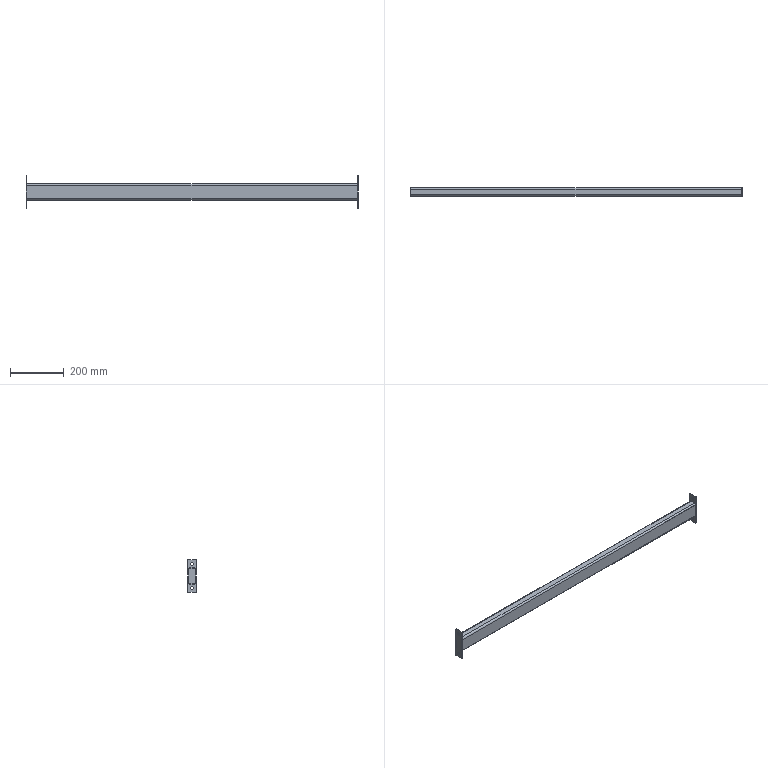Part | SolidWorks | features ICE 1, MirrorSolid 1, WeldMemberFeat 1, WeldmentFeature 1 | 3 solids | 38 faces | box 1240 x 30 x 120 mm | volume 613897 mm3 | plane 22 | cylinder 16 | commonest cylinder face diameters 10.5 x8 6 x4 12 x4
STEP:
#1=CARTESIAN_POINT('',(-617.,15.,24.));
#2=VERTEX_POINT('',#1);
#3=CARTESIAN_POINT('',(-617.,9.,30.));
#4=VERTEX_POINT('',#3);
#5=CARTESIAN_POINT('',(-617.,9.,24.));
#6=DIRECTION('',(1.,0.,0.));
#7=DIRECTION('',(0.,0.,-1.));
#8=AXIS2_PLACEMENT_3D('',#5,#6,#7);
#9=CIRCLE('',#8,6.);
#10=EDGE_CURVE('',#2,#4,#9,.T.);
#11=ORIENTED_EDGE('',*,*,#10,.T.);
#12=CARTESIAN_POINT('',(617.,9.,30.));
#13=VERTEX_POINT('',#12);
#14=CARTESIAN_POINT('',(617.,9.,30.));
#15=DIRECTION('',(-1.,0.,0.));
#16=VECTOR('',#15,1000.);
#17=LINE('',#14,#16);
#18=EDGE_CURVE('',#13,#4,#17,.T.);
#19=ORIENTED_EDGE('',*,*,#18,.F.);
#20=CARTESIAN_POINT('',(617.,15.,24.));
#21=VERTEX_POINT('',#20);
#22=CARTESIAN_POINT('',(617.,9.,24.));
#23=DIRECTION('',(1.,0.,0.));
#24=DIRECTION('',(0.,0.,-1.));
#25=AXIS2_PLACEMENT_3D('',#22,#23,#24);
#26=CIRCLE('',#25,6.);
#27=EDGE_CURVE('',#21,#13,#26,.T.);
#28=ORIENTED_EDGE('',*,*,#27,.F.);
#29=CARTESIAN_POINT('',(617.,15.,24.));
#30=DIRECTION('',(-1.,0.,0.));
#31=VECTOR('',#30,1000.);
#32=LINE('',#29,#31);
#33=EDGE_CURVE('',#21,#2,#32,.T.);
#34=ORIENTED_EDGE('',*,*,#33,.T.);
#35=EDGE_LOOP('',(#11,#19,#28,#34));
#36=FACE_OUTER_BOUND('',#35,.T.);
#37=CARTESIAN_POINT('',(617.,9.,24.));
#38=DIRECTION('',(-1.,0.,0.));
#39=DIRECTION('',(0.,0.,1.));
#40=AXIS2_PLACEMENT_3D('',#37,#38,#39);
#41=CYLINDRICAL_SURFACE('',#40,6.);
#42=ADVANCED_FACE('',(#36),#41,.T.);
#43=CARTESIAN_POINT('',(-617.,-9.,30.));
#44=VERTEX_POINT('',#43);
#45=CARTESIAN_POINT('',(-617.,9.,30.));
#46=DIRECTION('',(0.,-1.,0.));
#47=VECTOR('',#46,1000.);
#48=LINE('',#45,#47);
#49=EDGE_CURVE('',#4,#44,#48,.T.);
#50=ORIENTED_EDGE('',*,*,#49,.T.);
#51=CARTESIAN_POINT('',(617.,-9.,30.));
#52=VERTEX_POINT('',#51);
#53=CARTESIAN_POINT('',(617.,-9.,30.));
#54=DIRECTION('',(-1.,0.,0.));
#55=VECTOR('',#54,1000.);
#56=LINE('',#53,#55);
#57=EDGE_CURVE('',#52,#44,#56,.T.);
#58=ORIENTED_EDGE('',*,*,#57,.F.);
#59=CARTESIAN_POINT('',(617.,9.,30.));
#60=DIRECTION('',(0.,-1.,0.));
#61=VECTOR('',#60,1000.);
#62=LINE('',#59,#61);
#63=EDGE_CURVE('',#13,#52,#62,.T.);
#64=ORIENTED_EDGE('',*,*,#63,.F.);
#65=ORIENTED_EDGE('',*,*,#18,.T.);
#66=EDGE_LOOP('',(#50,#58,#64,#65));
#67=FACE_OUTER_BOUND('',#66,.T.);
#68=CARTESIAN_POINT('',(617.,9.,30.));
#69=DIRECTION('',(0.,0.,-1.));
#70=DIRECTION('',(-1.,0.,0.));
#71=AXIS2_PLACEMENT_3D('',#68,#69,#70);
#72=PLANE('',#71);
#73=ADVANCED_FACE('',(#67),#72,.F.);
#74=CARTESIAN_POINT('',(-617.,-15.,24.));
#75=VERTEX_POINT('',#74);
#76=CARTESIAN_POINT('',(-617.,-9.,24.));
#77=DIRECTION('',(1.,0.,0.));
#78=DIRECTION('',(0.,0.,-1.));
#79=AXIS2_PLACEMENT_3D('',#76,#77,#78);
#80=CIRCLE('',#79,6.);
#81=EDGE_CURVE('',#44,#75,#80,.T.);
#82=ORIENTED_EDGE('',*,*,#81,.T.);
#83=CARTESIAN_POINT('',(617.,-15.,24.));
#84=VERTEX_POINT('',#83);
#85=CARTESIAN_POINT('',(617.,-15.,24.));
#86=DIRECTION('',(-1.,0.,0.));
#87=VECTOR('',#86,1000.);
#88=LINE('',#85,#87);
#89=EDGE_CURVE('',#84,#75,#88,.T.);
#90=ORIENTED_EDGE('',*,*,#89,.F.);
#91=CARTESIAN_POINT('',(617.,-9.,24.));
#92=DIRECTION('',(1.,0.,0.));
#93=DIRECTION('',(0.,0.,-1.));
#94=AXIS2_PLACEMENT_3D('',#91,#92,#93);
#95=CIRCLE('',#94,6.);
#96=EDGE_CURVE('',#52,#84,#95,.T.);
#97=ORIENTED_EDGE('',*,*,#96,.F.);
#98=ORIENTED_EDGE('',*,*,#57,.T.);
#99=EDGE_LOOP('',(#82,#90,#97,#98));
#100=FACE_OUTER_BOUND('',#99,.T.);
#101=CARTESIAN_POINT('',(617.,-9.,24.));
#102=DIRECTION('',(-1.,0.,0.));
#103=DIRECTION('',(0.,0.,1.));
#104=AXIS2_PLACEMENT_3D('',#101,#102,#103);
#105=CYLINDRICAL_SURFACE('',#104,6.);
#106=ADVANCED_FACE('',(#100),#105,.T.);
#107=CARTESIAN_POINT('',(-617.,-15.,-24.));
#108=VERTEX_POINT('',#107);
#109=CARTESIAN_POINT('',(-617.,-15.,-24.));
#110=DIRECTION('',(0.,0.,-1.));
#111=VECTOR('',#110,1000.);
#112=LINE('',#109,#111);
#113=EDGE_CURVE('',#75,#108,#112,.T.);
#114=ORIENTED_EDGE('',*,*,#113,.T.);
#115=CARTESIAN_POINT('',(617.,-15.,-24.));
#116=VERTEX_POINT('',#115);
#117=CARTESIAN_POINT('',(617.,-15.,-24.));
#118=DIRECTION('',(-1.,0.,0.));
#119=VECTOR('',#118,1000.);
#120=LINE('',#117,#119);
#121=EDGE_CURVE('',#116,#108,#120,.T.);
#122=ORIENTED_EDGE('',*,*,#121,.F.);
#123=CARTESIAN_POINT('',(617.,-15.,-24.));
#124=DIRECTION('',(0.,0.,-1.));
#125=VECTOR('',#124,1000.);
#126=LINE('',#123,#125);
#127=EDGE_CURVE('',#84,#116,#126,.T.);
#128=ORIENTED_EDGE('',*,*,#127,.F.);
#129=ORIENTED_EDGE('',*,*,#89,.T.);
#130=EDGE_LOOP('',(#114,#122,#128,#129));
#131=FACE_OUTER_BOUND('',#130,.T.);
#132=CARTESIAN_POINT('',(617.,-15.,-24.));
#133=DIRECTION('',(0.,1.,0.));
#134=DIRECTION('',(0.,0.,1.));
#135=AXIS2_PLACEMENT_3D('',#132,#133,#134);
#136=PLANE('',#135);
#137=ADVANCED_FACE('',(#131),#136,.F.);
#138=CARTESIAN_POINT('',(-617.,-9.,-30.));
#139=VERTEX_POINT('',#138);
#140=CARTESIAN_POINT('',(-617.,-9.,-24.));
#141=DIRECTION('',(1.,0.,0.));
#142=DIRECTION('',(0.,0.,-1.));
#143=AXIS2_PLACEMENT_3D('',#140,#141,#142);
#144=CIRCLE('',#143,6.);
#145=EDGE_CURVE('',#108,#139,#144,.T.);
#146=ORIENTED_EDGE('',*,*,#145,.T.);
#147=CARTESIAN_POINT('',(617.,-9.,-30.));
#148=VERTEX_POINT('',#147);
#149=CARTESIAN_POINT('',(617.,-9.,-30.));
#150=DIRECTION('',(-1.,0.,0.));
#151=VECTOR('',#150,1000.);
#152=LINE('',#149,#151);
#153=EDGE_CURVE('',#148,#139,#152,.T.);
#154=ORIENTED_EDGE('',*,*,#153,.F.);
#155=CARTESIAN_POINT('',(617.,-9.,-24.));
#156=DIRECTION('',(1.,0.,0.));
#157=DIRECTION('',(0.,0.,-1.));
#158=AXIS2_PLACEMENT_3D('',#155,#156,#157);
#159=CIRCLE('',#158,6.);
#160=EDGE_CURVE('',#116,#148,#159,.T.);
#161=ORIENTED_EDGE('',*,*,#160,.F.);
#162=ORIENTED_EDGE('',*,*,#121,.T.);
#163=EDGE_LOOP('',(#146,#154,#161,#162));
#164=FACE_OUTER_BOUND('',#163,.T.);
#165=CARTESIAN_POINT('',(617.,-9.,-24.));
#166=DIRECTION('',(-1.,0.,0.));
#167=DIRECTION('',(0.,0.,1.));
#168=AXIS2_PLACEMENT_3D('',#165,#166,#167);
#169=CYLINDRICAL_SURFACE('',#168,6.);
#170=ADVANCED_FACE('',(#164),#169,.T.);
#171=CARTESIAN_POINT('',(-617.,9.,-30.));
#172=VERTEX_POINT('',#171);
#173=CARTESIAN_POINT('',(-617.,-9.,-30.));
#174=DIRECTION('',(0.,1.,0.));
#175=VECTOR('',#174,1000.);
#176=LINE('',#173,#175);
#177=EDGE_CURVE('',#139,#172,#176,.T.);
#178=ORIENTED_EDGE('',*,*,#177,.T.);
#179=CARTESIAN_POINT('',(617.,9.,-30.));
#180=VERTEX_POINT('',#179);
#181=CARTESIAN_POINT('',(617.,9.,-30.));
#182=DIRECTION('',(-1.,0.,0.));
#183=VECTOR('',#182,1000.);
#184=LINE('',#181,#183);
#185=EDGE_CURVE('',#180,#172,#184,.T.);
#186=ORIENTED_EDGE('',*,*,#185,.F.);
#187=CARTESIAN_POINT('',(617.,-9.,-30.));
#188=DIRECTION('',(0.,1.,0.));
#189=VECTOR('',#188,1000.);
#190=LINE('',#187,#189);
#191=EDGE_CURVE('',#148,#180,#190,.T.);
#192=ORIENTED_EDGE('',*,*,#191,.F.);
#193=ORIENTED_EDGE('',*,*,#153,.T.);
#194=EDGE_LOOP('',(#178,#186,#192,#193));
#195=FACE_OUTER_BOUND('',#194,.T.);
#196=CARTESIAN_POINT('',(617.,-9.,-30.));
#197=DIRECTION('',(0.,0.,1.));
#198=DIRECTION('',(1.,0.,0.));
#199=AXIS2_PLACEMENT_3D('',#196,#197,#198);
#200=PLANE('',#199);
#201=ADVANCED_FACE('',(#195),#200,.F.);
#202=CARTESIAN_POINT('',(-617.,15.,-24.));
#203=VERTEX_POINT('',#202);
#204=CARTESIAN_POINT('',(-617.,9.,-24.));
#205=DIRECTION('',(1.,0.,0.));
#206=DIRECTION('',(0.,0.,-1.));
#207=AXIS2_PLACEMENT_3D('',#204,#205,#206);
#208=CIRCLE('',#207,6.);
#209=EDGE_CURVE('',#172,#203,#208,.T.);
#210=ORIENTED_EDGE('',*,*,#209,.T.);
#211=CARTESIAN_POINT('',(617.,15.,-24.));
#212=VERTEX_POINT('',#211);
#213=CARTESIAN_POINT('',(617.,15.,-24.));
#214=DIRECTION('',(-1.,0.,0.));
#215=VECTOR('',#214,1000.);
#216=LINE('',#213,#215);
#217=EDGE_CURVE('',#212,#203,#216,.T.);
#218=ORIENTED_EDGE('',*,*,#217,.F.);
#219=CARTESIAN_POINT('',(617.,9.,-24.));
#220=DIRECTION('',(1.,0.,0.));
#221=DIRECTION('',(0.,0.,-1.));
#222=AXIS2_PLACEMENT_3D('',#219,#220,#221);
#223=CIRCLE('',#222,6.);
#224=EDGE_CURVE('',#180,#212,#223,.T.);
#225=ORIENTED_EDGE('',*,*,#224,.F.);
#226=ORIENTED_EDGE('',*,*,#185,.T.);
#227=EDGE_LOOP('',(#210,#218,#225,#226));
#228=FACE_OUTER_BOUND('',#227,.T.);
#229=CARTESIAN_POINT('',(617.,9.,-24.));
#230=DIRECTION('',(-1.,0.,0.));
#231=DIRECTION('',(0.,0.,1.));
#232=AXIS2_PLACEMENT_3D('',#229,#230,#231);
#233=CYLINDRICAL_SURFACE('',#232,6.);
#234=ADVANCED_FACE('',(#228),#233,.T.);
#235=CARTESIAN_POINT('',(-617.,-9.,27.));
#236=VERTEX_POINT('',#235);
#237=CARTESIAN_POINT('',(-617.,-12.,24.));
#238=VERTEX_POINT('',#237);
#239=CARTESIAN_POINT('',(-617.,-9.,24.));
#240=DIRECTION('',(1.,0.,0.));
#241=DIRECTION('',(0.,0.,-1.));
#242=AXIS2_PLACEMENT_3D('',#239,#240,#241);
#243=CIRCLE('',#242,3.);
#244=EDGE_CURVE('',#236,#238,#243,.T.);
#245=ORIENTED_EDGE('',*,*,#244,.F.);
#246=CARTESIAN_POINT('',(617.,-9.,27.));
#247=VERTEX_POINT('',#246);
#248=CARTESIAN_POINT('',(617.,-9.,27.));
#249=DIRECTION('',(-1.,0.,0.));
#250=VECTOR('',#249,1000.);
#251=LINE('',#248,#250);
#252=EDGE_CURVE('',#247,#236,#251,.T.);
#253=ORIENTED_EDGE('',*,*,#252,.F.);
#254=CARTESIAN_POINT('',(617.,-12.,24.));
#255=VERTEX_POINT('',#254);
#256=CARTESIAN_POINT('',(617.,-9.,24.));
#257=DIRECTION('',(1.,0.,0.));
#258=DIRECTION('',(0.,0.,-1.));
#259=AXIS2_PLACEMENT_3D('',#256,#257,#258);
#260=CIRCLE('',#259,3.);
#261=EDGE_CURVE('',#247,#255,#260,.T.);
#262=ORIENTED_EDGE('',*,*,#261,.T.);
#263=CARTESIAN_POINT('',(617.,-12.,24.));
#264=DIRECTION('',(-1.,0.,0.));
#265=VECTOR('',#264,1000.);
#266=LINE('',#263,#265);
#267=EDGE_CURVE('',#255,#238,#266,.T.);
#268=ORIENTED_EDGE('',*,*,#267,.T.);
#269=EDGE_LOOP('',(#245,#253,#262,#268));
#270=FACE_OUTER_BOUND('',#269,.T.);
#271=CARTESIAN_POINT('',(617.,-9.,24.));
#272=DIRECTION('',(-1.,0.,0.));
#273=DIRECTION('',(0.,0.,1.));
#274=AXIS2_PLACEMENT_3D('',#271,#272,#273);
#275=CYLINDRICAL_SURFACE('',#274,3.);
#276=ADVANCED_FACE('',(#270),#275,.F.);
#277=CARTESIAN_POINT('',(-617.,9.,27.));
#278=VERTEX_POINT('',#277);
#279=CARTESIAN_POINT('',(-617.,9.,27.));
#280=DIRECTION('',(0.,-1.,0.));
#281=VECTOR('',#280,1000.);
#282=LINE('',#279,#281);
#283=EDGE_CURVE('',#278,#236,#282,.T.);
#284=ORIENTED_EDGE('',*,*,#283,.F.);
#285=CARTESIAN_POINT('',(617.,9.,27.));
#286=VERTEX_POINT('',#285);
#287=CARTESIAN_POINT('',(617.,9.,27.));
#288=DIRECTION('',(-1.,0.,0.));
#289=VECTOR('',#288,1000.);
#290=LINE('',#287,#289);
#291=EDGE_CURVE('',#286,#278,#290,.T.);
#292=ORIENTED_EDGE('',*,*,#291,.F.);
#293=CARTESIAN_POINT('',(617.,9.,27.));
#294=DIRECTION('',(0.,-1.,0.));
#295=VECTOR('',#294,1000.);
#296=LINE('',#293,#295);
#297=EDGE_CURVE('',#286,#247,#296,.T.);
#298=ORIENTED_EDGE('',*,*,#297,.T.);
#299=ORIENTED_EDGE('',*,*,#252,.T.);
#300=EDGE_LOOP('',(#284,#292,#298,#299));
#301=FACE_OUTER_BOUND('',#300,.T.);
#302=CARTESIAN_POINT('',(617.,9.,27.));
#303=DIRECTION('',(0.,0.,-1.));
#304=DIRECTION('',(-1.,0.,0.));
#305=AXIS2_PLACEMENT_3D('',#302,#303,#304);
#306=PLANE('',#305);
#307=ADVANCED_FACE('',(#301),#306,.T.);
#308=CARTESIAN_POINT('',(-617.,12.,24.));
#309=VERTEX_POINT('',#308);
#310=CARTESIAN_POINT('',(-617.,9.,24.));
#311=DIRECTION('',(1.,0.,0.));
#312=DIRECTION('',(0.,0.,-1.));
#313=AXIS2_PLACEMENT_3D('',#310,#311,#312);
#314=CIRCLE('',#313,3.);
#315=EDGE_CURVE('',#309,#278,#314,.T.);
#316=ORIENTED_EDGE('',*,*,#315,.F.);
#317=CARTESIAN_POINT('',(617.,12.,24.));
#318=VERTEX_POINT('',#317);
#319=CARTESIAN_POINT('',(617.,12.,24.));
#320=DIRECTION('',(-1.,0.,0.));
#321=VECTOR('',#320,1000.);
#322=LINE('',#319,#321);
#323=EDGE_CURVE('',#318,#309,#322,.T.);
#324=ORIENTED_EDGE('',*,*,#323,.F.);
#325=CARTESIAN_POINT('',(617.,9.,24.));
#326=DIRECTION('',(1.,0.,0.));
#327=DIRECTION('',(0.,0.,-1.));
#328=AXIS2_PLACEMENT_3D('',#325,#326,#327);
#329=CIRCLE('',#328,3.);
#330=EDGE_CURVE('',#318,#286,#329,.T.);
#331=ORIENTED_EDGE('',*,*,#330,.T.);
#332=ORIENTED_EDGE('',*,*,#291,.T.);
#333=EDGE_LOOP('',(#316,#324,#331,#332));
#334=FACE_OUTER_BOUND('',#333,.T.);
#335=CARTESIAN_POINT('',(617.,9.,24.));
#336=DIRECTION('',(-1.,0.,0.));
#337=DIRECTION('',(0.,0.,1.));
#338=AXIS2_PLACEMENT_3D('',#335,#336,#337);
#339=CYLINDRICAL_SURFACE('',#338,3.);
#340=ADVANCED_FACE('',(#334),#339,.F.);
#341=CARTESIAN_POINT('',(-617.,12.,-24.));
#342=VERTEX_POINT('',#341);
#343=CARTESIAN_POINT('',(-617.,12.,24.));
#344=DIRECTION('',(0.,0.,1.));
#345=VECTOR('',#344,1000.);
#346=LINE('',#343,#345);
#347=EDGE_CURVE('',#342,#309,#346,.T.);
#348=ORIENTED_EDGE('',*,*,#347,.F.);
#349=CARTESIAN_POINT('',(617.,12.,-24.));
#350=VERTEX_POINT('',#349);
#351=CARTESIAN_POINT('',(617.,12.,-24.));
#352=DIRECTION('',(-1.,0.,0.));
#353=VECTOR('',#352,1000.);
#354=LINE('',#351,#353);
#355=EDGE_CURVE('',#350,#342,#354,.T.);
#356=ORIENTED_EDGE('',*,*,#355,.F.);
#357=CARTESIAN_POINT('',(617.,12.,24.));
#358=DIRECTION('',(0.,0.,1.));
#359=VECTOR('',#358,1000.);
#360=LINE('',#357,#359);
#361=EDGE_CURVE('',#350,#318,#360,.T.);
#362=ORIENTED_EDGE('',*,*,#361,.T.);
#363=ORIENTED_EDGE('',*,*,#323,.T.);
#364=EDGE_LOOP('',(#348,#356,#362,#363));
#365=FACE_OUTER_BOUND('',#364,.T.);
#366=CARTESIAN_POINT('',(617.,12.,24.));
#367=DIRECTION('',(0.,-1.,0.));
#368=DIRECTION('',(0.,0.,-1.));
#369=AXIS2_PLACEMENT_3D('',#366,#367,#368);
#370=PLANE('',#369);
#371=ADVANCED_FACE('',(#365),#370,.T.);
#372=CARTESIAN_POINT('',(-617.,9.,-27.));
#373=VERTEX_POINT('',#372);
#374=CARTESIAN_POINT('',(-617.,9.,-24.));
#375=DIRECTION('',(1.,0.,0.));
#376=DIRECTION('',(0.,0.,-1.));
#377=AXIS2_PLACEMENT_3D('',#374,#375,#376);
#378=CIRCLE('',#377,3.);
#379=EDGE_CURVE('',#373,#342,#378,.T.);
#380=ORIENTED_EDGE('',*,*,#379,.F.);
#381=CARTESIAN_POINT('',(617.,9.,-27.));
#382=VERTEX_POINT('',#381);
#383=CARTESIAN_POINT('',(617.,9.,-27.));
#384=DIRECTION('',(-1.,0.,0.));
#385=VECTOR('',#384,1000.);
#386=LINE('',#383,#385);
#387=EDGE_CURVE('',#382,#373,#386,.T.);
#388=ORIENTED_EDGE('',*,*,#387,.F.);
#389=CARTESIAN_POINT('',(617.,9.,-24.));
#390=DIRECTION('',(1.,0.,0.));
#391=DIRECTION('',(0.,0.,-1.));
#392=AXIS2_PLACEMENT_3D('',#389,#390,#391);
#393=CIRCLE('',#392,3.);
#394=EDGE_CURVE('',#382,#350,#393,.T.);
#395=ORIENTED_EDGE('',*,*,#394,.T.);
#396=ORIENTED_EDGE('',*,*,#355,.T.);
#397=EDGE_LOOP('',(#380,#388,#395,#396));
#398=FACE_OUTER_BOUND('',#397,.T.);
#399=CARTESIAN_POINT('',(617.,9.,-24.));
#400=DIRECTION('',(-1.,0.,0.));
#401=DIRECTION('',(0.,0.,1.));
#402=AXIS2_PLACEMENT_3D('',#399,#400,#401);
#403=CYLINDRICAL_SURFACE('',#402,3.);
#404=ADVANCED_FACE('',(#398),#403,.F.);
#405=CARTESIAN_POINT('',(-617.,-9.,-27.));
#406=VERTEX_POINT('',#405);
#407=CARTESIAN_POINT('',(-617.,-9.,-27.));
#408=DIRECTION('',(0.,1.,0.));
#409=VECTOR('',#408,1000.);
#410=LINE('',#407,#409);
#411=EDGE_CURVE('',#406,#373,#410,.T.);
#412=ORIENTED_EDGE('',*,*,#411,.F.);
#413=CARTESIAN_POINT('',(617.,-9.,-27.));
#414=VERTEX_POINT('',#413);
#415=CARTESIAN_POINT('',(617.,-9.,-27.));
#416=DIRECTION('',(-1.,0.,0.));
#417=VECTOR('',#416,1000.);
#418=LINE('',#415,#417);
#419=EDGE_CURVE('',#414,#406,#418,.T.);
#420=ORIENTED_EDGE('',*,*,#419,.F.);
#421=CARTESIAN_POINT('',(617.,-9.,-27.));
#422=DIRECTION('',(0.,1.,0.));
#423=VECTOR('',#422,1000.);
#424=LINE('',#421,#423);
#425=EDGE_CURVE('',#414,#382,#424,.T.);
#426=ORIENTED_EDGE('',*,*,#425,.T.);
#427=ORIENTED_EDGE('',*,*,#387,.T.);
#428=EDGE_LOOP('',(#412,#420,#426,#427));
#429=FACE_OUTER_BOUND('',#428,.T.);
#430=CARTESIAN_POINT('',(617.,-9.,-27.));
#431=DIRECTION('',(0.,0.,1.));
#432=DIRECTION('',(1.,0.,0.));
#433=AXIS2_PLACEMENT_3D('',#430,#431,#432);
#434=PLANE('',#433);
#435=ADVANCED_FACE('',(#429),#434,.T.);
#436=CARTESIAN_POINT('',(-617.,-12.,-24.));
#437=VERTEX_POINT('',#436);
#438=CARTESIAN_POINT('',(-617.,-9.,-24.));
#439=DIRECTION('',(1.,0.,0.));
#440=DIRECTION('',(0.,0.,-1.));
#441=AXIS2_PLACEMENT_3D('',#438,#439,#440);
#442=CIRCLE('',#441,3.);
#443=EDGE_CURVE('',#437,#406,#442,.T.);
#444=ORIENTED_EDGE('',*,*,#443,.F.);
#445=CARTESIAN_POINT('',(617.,-12.,-24.));
#446=VERTEX_POINT('',#445);
#447=CARTESIAN_POINT('',(617.,-12.,-24.));
#448=DIRECTION('',(-1.,0.,0.));
#449=VECTOR('',#448,1000.);
#450=LINE('',#447,#449);
#451=EDGE_CURVE('',#446,#437,#450,.T.);
#452=ORIENTED_EDGE('',*,*,#451,.F.);
#453=CARTESIAN_POINT('',(617.,-9.,-24.));
#454=DIRECTION('',(1.,0.,0.));
#455=DIRECTION('',(0.,0.,-1.));
#456=AXIS2_PLACEMENT_3D('',#453,#454,#455);
#457=CIRCLE('',#456,3.);
#458=EDGE_CURVE('',#446,#414,#457,.T.);
#459=ORIENTED_EDGE('',*,*,#458,.T.);
#460=ORIENTED_EDGE('',*,*,#419,.T.);
#461=EDGE_LOOP('',(#444,#452,#459,#460));
#462=FACE_OUTER_BOUND('',#461,.T.);
#463=CARTESIAN_POINT('',(617.,-9.,-24.));
#464=DIRECTION('',(-1.,0.,0.));
#465=DIRECTION('',(0.,0.,1.));
#466=AXIS2_PLACEMENT_3D('',#463,#464,#465);
#467=CYLINDRICAL_SURFACE('',#466,3.);
#468=ADVANCED_FACE('',(#462),#467,.F.);
#469=CARTESIAN_POINT('',(-617.,-12.,-24.));
#470=DIRECTION('',(0.,0.,-1.));
#471=VECTOR('',#470,1000.);
#472=LINE('',#469,#471);
#473=EDGE_CURVE('',#238,#437,#472,.T.);
#474=ORIENTED_EDGE('',*,*,#473,.F.);
#475=ORIENTED_EDGE('',*,*,#267,.F.);
#476=CARTESIAN_POINT('',(617.,-12.,-24.));
#477=DIRECTION('',(0.,0.,-1.));
#478=VECTOR('',#477,1000.);
#479=LINE('',#476,#478);
#480=EDGE_CURVE('',#255,#446,#479,.T.);
#481=ORIENTED_EDGE('',*,*,#480,.T.);
#482=ORIENTED_EDGE('',*,*,#451,.T.);
#483=EDGE_LOOP('',(#474,#475,#481,#482));
#484=FACE_OUTER_BOUND('',#483,.T.);
#485=CARTESIAN_POINT('',(617.,-12.,-24.));
#486=DIRECTION('',(0.,1.,0.));
#487=DIRECTION('',(0.,0.,1.));
#488=AXIS2_PLACEMENT_3D('',#485,#486,#487);
#489=PLANE('',#488);
#490=ADVANCED_FACE('',(#484),#489,.T.);
#491=CARTESIAN_POINT('',(-617.,15.,24.));
#492=DIRECTION('',(0.,0.,1.));
#493=VECTOR('',#492,1000.);
#494=LINE('',#491,#493);
#495=EDGE_CURVE('',#203,#2,#494,.T.);
#496=ORIENTED_EDGE('',*,*,#495,.T.);
#497=ORIENTED_EDGE('',*,*,#33,.F.);
#498=CARTESIAN_POINT('',(617.,15.,24.));
#499=DIRECTION('',(0.,0.,1.));
#500=VECTOR('',#499,1000.);
#501=LINE('',#498,#500);
#502=EDGE_CURVE('',#212,#21,#501,.T.);
#503=ORIENTED_EDGE('',*,*,#502,.F.);
#504=ORIENTED_EDGE('',*,*,#217,.T.);
#505=EDGE_LOOP('',(#496,#497,#503,#504));
#506=FACE_OUTER_BOUND('',#505,.T.);
#507=CARTESIAN_POINT('',(617.,15.,24.));
#508=DIRECTION('',(0.,-1.,0.));
#509=DIRECTION('',(0.,0.,-1.));
#510=AXIS2_PLACEMENT_3D('',#507,#508,#509);
#511=PLANE('',#510);
#512=ADVANCED_FACE('',(#506),#511,.F.);
#513=ORIENTED_EDGE('',*,*,#261,.F.);
#514=ORIENTED_EDGE('',*,*,#297,.F.);
#515=ORIENTED_EDGE('',*,*,#330,.F.);
#516=ORIENTED_EDGE('',*,*,#361,.F.);
#517=ORIENTED_EDGE('',*,*,#394,.F.);
#518=ORIENTED_EDGE('',*,*,#425,.F.);
#519=ORIENTED_EDGE('',*,*,#458,.F.);
#520=ORIENTED_EDGE('',*,*,#480,.F.);
#521=EDGE_LOOP('',(#513,#514,#515,#516,#517,#518,#519,#520));
#522=FACE_BOUND('',#521,.T.);
#523=ORIENTED_EDGE('',*,*,#27,.T.);
#524=ORIENTED_EDGE('',*,*,#63,.T.);
#525=ORIENTED_EDGE('',*,*,#96,.T.);
#526=ORIENTED_EDGE('',*,*,#127,.T.);
#527=ORIENTED_EDGE('',*,*,#160,.T.);
#528=ORIENTED_EDGE('',*,*,#191,.T.);
#529=ORIENTED_EDGE('',*,*,#224,.T.);
#530=ORIENTED_EDGE('',*,*,#502,.T.);
#531=EDGE_LOOP('',(#523,#524,#525,#526,#527,#528,#529,#530));
#532=FACE_OUTER_BOUND('',#531,.T.);
#533=CARTESIAN_POINT('',(617.,9.,24.));
#534=DIRECTION('',(1.,0.,0.));
#535=DIRECTION('',(0.,0.,-1.));
#536=AXIS2_PLACEMENT_3D('',#533,#534,#535);
#537=PLANE('',#536);
#538=ADVANCED_FACE('',(#522,#532),#537,.T.);
#539=ORIENTED_EDGE('',*,*,#244,.T.);
#540=ORIENTED_EDGE('',*,*,#473,.T.);
#541=ORIENTED_EDGE('',*,*,#443,.T.);
#542=ORIENTED_EDGE('',*,*,#411,.T.);
#543=ORIENTED_EDGE('',*,*,#379,.T.);
#544=ORIENTED_EDGE('',*,*,#347,.T.);
#545=ORIENTED_EDGE('',*,*,#315,.T.);
#546=ORIENTED_EDGE('',*,*,#283,.T.);
#547=EDGE_LOOP('',(#539,#540,#541,#542,#543,#544,#545,#546));
#548=FACE_BOUND('',#547,.T.);
#549=ORIENTED_EDGE('',*,*,#10,.F.);
#550=ORIENTED_EDGE('',*,*,#495,.F.);
#551=ORIENTED_EDGE('',*,*,#209,.F.);
#552=ORIENTED_EDGE('',*,*,#177,.F.);
#553=ORIENTED_EDGE('',*,*,#145,.F.);
#554=ORIENTED_EDGE('',*,*,#113,.F.);
#555=ORIENTED_EDGE('',*,*,#81,.F.);
#556=ORIENTED_EDGE('',*,*,#49,.F.);
#557=EDGE_LOOP('',(#549,#550,#551,#552,#553,#554,#555,#556));
#558=FACE_OUTER_BOUND('',#557,.T.);
#559=CARTESIAN_POINT('',(-617.,9.,24.));
#560=DIRECTION('',(1.,0.,0.));
#561=DIRECTION('',(0.,0.,-1.));
#562=AXIS2_PLACEMENT_3D('',#559,#560,#561);
#563=PLANE('',#562);
#564=ADVANCED_FACE('',(#548,#558),#563,.F.);
#565=CLOSED_SHELL('',(#42,#73,#106,#137,#170,#201,#234,#276,#307,#340,#371,#404,#435,#468,#490,#512,#538,#564));
#566=MANIFOLD_SOLID_BREP('',#565);
#567=CARTESIAN_POINT('',(620.,0.,50.25));
#568=VERTEX_POINT('',#567);
#569=CARTESIAN_POINT('',(620.,0.,39.75));
#570=VERTEX_POINT('',#569);
#571=CARTESIAN_POINT('',(620.,0.,45.));
#572=DIRECTION('',(1.,0.,0.));
#573=DIRECTION('',(0.,0.,1.));
#574=AXIS2_PLACEMENT_3D('',#571,#572,#573);
#575=CIRCLE('',#574,5.25);
#576=EDGE_CURVE('',#568,#570,#575,.T.);
#577=ORIENTED_EDGE('',*,*,#576,.T.);
#578=CARTESIAN_POINT('',(617.,0.,39.75));
#579=VERTEX_POINT('',#578);
#580=CARTESIAN_POINT('',(620.,0.,39.75));
#581=DIRECTION('',(-1.,0.,0.));
#582=VECTOR('',#581,1000.);
#583=LINE('',#580,#582);
#584=EDGE_CURVE('',#570,#579,#583,.T.);
#585=ORIENTED_EDGE('',*,*,#584,.T.);
#586=CARTESIAN_POINT('',(617.,0.,50.25));
#587=VERTEX_POINT('',#586);
#588=CARTESIAN_POINT('',(617.,0.,45.));
#589=DIRECTION('',(1.,0.,0.));
#590=DIRECTION('',(0.,0.,1.));
#591=AXIS2_PLACEMENT_3D('',#588,#589,#590);
#592=CIRCLE('',#591,5.25);
#593=EDGE_CURVE('',#587,#579,#592,.T.);
#594=ORIENTED_EDGE('',*,*,#593,.F.);
#595=CARTESIAN_POINT('',(620.,0.,50.25));
#596=DIRECTION('',(-1.,0.,0.));
#597=VECTOR('',#596,1000.);
#598=LINE('',#595,#597);
#599=EDGE_CURVE('',#568,#587,#598,.T.);
#600=ORIENTED_EDGE('',*,*,#599,.F.);
#601=EDGE_LOOP('',(#577,#585,#594,#600));
#602=FACE_OUTER_BOUND('',#601,.T.);
#603=CARTESIAN_POINT('',(620.,0.,45.));
#604=DIRECTION('',(-1.,0.,0.));
#605=DIRECTION('',(0.,0.,1.));
#606=AXIS2_PLACEMENT_3D('',#603,#604,#605);
#607=CYLINDRICAL_SURFACE('',#606,5.25);
#608=ADVANCED_FACE('',(#602),#607,.F.);
#609=CARTESIAN_POINT('',(620.,0.,-39.75));
#610=VERTEX_POINT('',#609);
#611=CARTESIAN_POINT('',(620.,0.,-50.25));
#612=VERTEX_POINT('',#611);
#613=CARTESIAN_POINT('',(620.,0.,-45.));
#614=DIRECTION('',(1.,0.,0.));
#615=DIRECTION('',(0.,0.,-1.));
#616=AXIS2_PLACEMENT_3D('',#613,#614,#615);
#617=CIRCLE('',#616,5.25);
#618=EDGE_CURVE('',#610,#612,#617,.T.);
#619=ORIENTED_EDGE('',*,*,#618,.T.);
#620=CARTESIAN_POINT('',(617.,0.,-50.25));
#621=VERTEX_POINT('',#620);
#622=CARTESIAN_POINT('',(620.,0.,-50.25));
#623=DIRECTION('',(-1.,0.,0.));
#624=VECTOR('',#623,1000.);
#625=LINE('',#622,#624);
#626=EDGE_CURVE('',#612,#621,#625,.T.);
#627=ORIENTED_EDGE('',*,*,#626,.T.);
#628=CARTESIAN_POINT('',(617.,0.,-39.75));
#629=VERTEX_POINT('',#628);
#630=CARTESIAN_POINT('',(617.,0.,-45.));
#631=DIRECTION('',(1.,0.,0.));
#632=DIRECTION('',(0.,0.,-1.));
#633=AXIS2_PLACEMENT_3D('',#630,#631,#632);
#634=CIRCLE('',#633,5.25);
#635=EDGE_CURVE('',#629,#621,#634,.T.);
#636=ORIENTED_EDGE('',*,*,#635,.F.);
#637=CARTESIAN_POINT('',(620.,0.,-39.75));
#638=DIRECTION('',(-1.,0.,0.));
#639=VECTOR('',#638,1000.);
#640=LINE('',#637,#639);
#641=EDGE_CURVE('',#610,#629,#640,.T.);
#642=ORIENTED_EDGE('',*,*,#641,.F.);
#643=EDGE_LOOP('',(#619,#627,#636,#642));
#644=FACE_OUTER_BOUND('',#643,.T.);
#645=CARTESIAN_POINT('',(620.,0.,-45.));
#646=DIRECTION('',(-1.,0.,0.));
#647=DIRECTION('',(0.,0.,1.));
#648=AXIS2_PLACEMENT_3D('',#645,#646,#647);
#649=CYLINDRICAL_SURFACE('',#648,5.25);
#650=ADVANCED_FACE('',(#644),#649,.F.);
#651=ORIENTED_EDGE('',*,*,#618,.F.);
#652=CARTESIAN_POINT('',(620.,0.,-45.));
#653=DIRECTION('',(1.,0.,0.));
#654=DIRECTION('',(0.,0.,-1.));
#655=AXIS2_PLACEMENT_3D('',#652,#653,#654);
#656=CIRCLE('',#655,5.25);
#657=EDGE_CURVE('',#612,#610,#656,.T.);
#658=ORIENTED_EDGE('',*,*,#657,.F.);
#659=EDGE_LOOP('',(#651,#658));
#660=FACE_BOUND('',#659,.T.);
#661=CARTESIAN_POINT('',(620.,-15.,-60.));
#662=VERTEX_POINT('',#661);
#663=CARTESIAN_POINT('',(620.,15.,-60.));
#664=VERTEX_POINT('',#663);
#665=CARTESIAN_POINT('',(620.,-15.,-60.));
#666=DIRECTION('',(0.,1.,0.));
#667=VECTOR('',#666,1000.);
#668=LINE('',#665,#667);
#669=EDGE_CURVE('',#662,#664,#668,.T.);
#670=ORIENTED_EDGE('',*,*,#669,.T.);
#671=CARTESIAN_POINT('',(620.,15.,60.));
#672=VERTEX_POINT('',#671);
#673=CARTESIAN_POINT('',(620.,15.,60.));
#674=DIRECTION('',(0.,0.,1.));
#675=VECTOR('',#674,1000.);
#676=LINE('',#673,#675);
#677=EDGE_CURVE('',#664,#672,#676,.T.);
#678=ORIENTED_EDGE('',*,*,#677,.T.);
#679=CARTESIAN_POINT('',(620.,-15.,60.));
#680=VERTEX_POINT('',#679);
#681=CARTESIAN_POINT('',(620.,-15.,60.));
#682=DIRECTION('',(0.,-1.,0.));
#683=VECTOR('',#682,1000.);
#684=LINE('',#681,#683);
#685=EDGE_CURVE('',#672,#680,#684,.T.);
#686=ORIENTED_EDGE('',*,*,#685,.T.);
#687=CARTESIAN_POINT('',(620.,-15.,60.));
#688=DIRECTION('',(0.,0.,-1.));
#689=VECTOR('',#688,1000.);
#690=LINE('',#687,#689);
#691=EDGE_CURVE('',#680,#662,#690,.T.);
#692=ORIENTED_EDGE('',*,*,#691,.T.);
#693=EDGE_LOOP('',(#670,#678,#686,#692));
#694=FACE_OUTER_BOUND('',#693,.T.);
#695=ORIENTED_EDGE('',*,*,#576,.F.);
#696=CARTESIAN_POINT('',(620.,0.,45.));
#697=DIRECTION('',(1.,0.,0.));
#698=DIRECTION('',(0.,0.,1.));
#699=AXIS2_PLACEMENT_3D('',#696,#697,#698);
#700=CIRCLE('',#699,5.25);
#701=EDGE_CURVE('',#570,#568,#700,.T.);
#702=ORIENTED_EDGE('',*,*,#701,.F.);
#703=EDGE_LOOP('',(#695,#702));
#704=FACE_BOUND('',#703,.T.);
#705=CARTESIAN_POINT('',(620.,0.,0.));
#706=DIRECTION('',(-1.,0.,0.));
#707=DIRECTION('',(0.,0.,1.));
#708=AXIS2_PLACEMENT_3D('',#705,#706,#707);
#709=PLANE('',#708);
#710=ADVANCED_FACE('',(#660,#694,#704),#709,.F.);
#711=ORIENTED_EDGE('',*,*,#635,.T.);
#712=CARTESIAN_POINT('',(617.,0.,-45.));
#713=DIRECTION('',(1.,0.,0.));
#714=DIRECTION('',(0.,0.,-1.));
#715=AXIS2_PLACEMENT_3D('',#712,#713,#714);
#716=CIRCLE('',#715,5.25);
#717=EDGE_CURVE('',#621,#629,#716,.T.);
#718=ORIENTED_EDGE('',*,*,#717,.T.);
#719=EDGE_LOOP('',(#711,#718));
#720=FACE_BOUND('',#719,.T.);
#721=CARTESIAN_POINT('',(617.,-15.,-60.));
#722=VERTEX_POINT('',#721);
#723=CARTESIAN_POINT('',(617.,15.,-60.));
#724=VERTEX_POINT('',#723);
#725=CARTESIAN_POINT('',(617.,-15.,-60.));
#726=DIRECTION('',(0.,1.,0.));
#727=VECTOR('',#726,1000.);
#728=LINE('',#725,#727);
#729=EDGE_CURVE('',#722,#724,#728,.T.);
#730=ORIENTED_EDGE('',*,*,#729,.F.);
#731=CARTESIAN_POINT('',(617.,-15.,60.));
#732=VERTEX_POINT('',#731);
#733=CARTESIAN_POINT('',(617.,-15.,60.));
#734=DIRECTION('',(0.,0.,-1.));
#735=VECTOR('',#734,1000.);
#736=LINE('',#733,#735);
#737=EDGE_CURVE('',#732,#722,#736,.T.);
#738=ORIENTED_EDGE('',*,*,#737,.F.);
#739=CARTESIAN_POINT('',(617.,15.,60.));
#740=VERTEX_POINT('',#739);
#741=CARTESIAN_POINT('',(617.,-15.,60.));
#742=DIRECTION('',(0.,-1.,0.));
#743=VECTOR('',#742,1000.);
#744=LINE('',#741,#743);
#745=EDGE_CURVE('',#740,#732,#744,.T.);
#746=ORIENTED_EDGE('',*,*,#745,.F.);
#747=CARTESIAN_POINT('',(617.,15.,60.));
#748=DIRECTION('',(0.,0.,1.));
#749=VECTOR('',#748,1000.);
#750=LINE('',#747,#749);
#751=EDGE_CURVE('',#724,#740,#750,.T.);
#752=ORIENTED_EDGE('',*,*,#751,.F.);
#753=EDGE_LOOP('',(#730,#738,#746,#752));
#754=FACE_OUTER_BOUND('',#753,.T.);
#755=ORIENTED_EDGE('',*,*,#593,.T.);
#756=CARTESIAN_POINT('',(617.,0.,45.));
#757=DIRECTION('',(1.,0.,0.));
#758=DIRECTION('',(0.,0.,1.));
#759=AXIS2_PLACEMENT_3D('',#756,#757,#758);
#760=CIRCLE('',#759,5.25);
#761=EDGE_CURVE('',#579,#587,#760,.T.);
#762=ORIENTED_EDGE('',*,*,#761,.T.);
#763=EDGE_LOOP('',(#755,#762));
#764=FACE_BOUND('',#763,.T.);
#765=CARTESIAN_POINT('',(617.,0.,0.));
#766=DIRECTION('',(-1.,0.,0.));
#767=DIRECTION('',(0.,0.,1.));
#768=AXIS2_PLACEMENT_3D('',#765,#766,#767);
#769=PLANE('',#768);
#770=ADVANCED_FACE('',(#720,#754,#764),#769,.T.);
#771=ORIENTED_EDGE('',*,*,#729,.T.);
#772=CARTESIAN_POINT('',(620.,15.,-60.));
#773=DIRECTION('',(-1.,0.,0.));
#774=VECTOR('',#773,1000.);
#775=LINE('',#772,#774);
#776=EDGE_CURVE('',#664,#724,#775,.T.);
#777=ORIENTED_EDGE('',*,*,#776,.F.);
#778=ORIENTED_EDGE('',*,*,#669,.F.);
#779=CARTESIAN_POINT('',(620.,-15.,-60.));
#780=DIRECTION('',(-1.,0.,0.));
#781=VECTOR('',#780,1000.);
#782=LINE('',#779,#781);
#783=EDGE_CURVE('',#662,#722,#782,.T.);
#784=ORIENTED_EDGE('',*,*,#783,.T.);
#785=EDGE_LOOP('',(#771,#777,#778,#784));
#786=FACE_OUTER_BOUND('',#785,.T.);
#787=CARTESIAN_POINT('',(620.,-15.,-60.));
#788=DIRECTION('',(0.,0.,1.));
#789=DIRECTION('',(1.,0.,0.));
#790=AXIS2_PLACEMENT_3D('',#787,#788,#789);
#791=PLANE('',#790);
#792=ADVANCED_FACE('',(#786),#791,.F.);
#793=ORIENTED_EDGE('',*,*,#751,.T.);
#794=CARTESIAN_POINT('',(620.,15.,60.));
#795=DIRECTION('',(-1.,0.,0.));
#796=VECTOR('',#795,1000.);
#797=LINE('',#794,#796);
#798=EDGE_CURVE('',#672,#740,#797,.T.);
#799=ORIENTED_EDGE('',*,*,#798,.F.);
#800=ORIENTED_EDGE('',*,*,#677,.F.);
#801=ORIENTED_EDGE('',*,*,#776,.T.);
#802=EDGE_LOOP('',(#793,#799,#800,#801));
#803=FACE_OUTER_BOUND('',#802,.T.);
#804=CARTESIAN_POINT('',(620.,15.,60.));
#805=DIRECTION('',(0.,-1.,0.));
#806=DIRECTION('',(0.,0.,-1.));
#807=AXIS2_PLACEMENT_3D('',#804,#805,#806);
#808=PLANE('',#807);
#809=ADVANCED_FACE('',(#803),#808,.F.);
#810=ORIENTED_EDGE('',*,*,#745,.T.);
#811=CARTESIAN_POINT('',(620.,-15.,60.));
#812=DIRECTION('',(-1.,0.,0.));
#813=VECTOR('',#812,1000.);
#814=LINE('',#811,#813);
#815=EDGE_CURVE('',#680,#732,#814,.T.);
#816=ORIENTED_EDGE('',*,*,#815,.F.);
#817=ORIENTED_EDGE('',*,*,#685,.F.);
#818=ORIENTED_EDGE('',*,*,#798,.T.);
#819=EDGE_LOOP('',(#810,#816,#817,#818));
#820=FACE_OUTER_BOUND('',#819,.T.);
#821=CARTESIAN_POINT('',(620.,-15.,60.));
#822=DIRECTION('',(0.,0.,-1.));
#823=DIRECTION('',(-1.,0.,0.));
#824=AXIS2_PLACEMENT_3D('',#821,#822,#823);
#825=PLANE('',#824);
#826=ADVANCED_FACE('',(#820),#825,.F.);
#827=ORIENTED_EDGE('',*,*,#737,.T.);
#828=ORIENTED_EDGE('',*,*,#783,.F.);
#829=ORIENTED_EDGE('',*,*,#691,.F.);
#830=ORIENTED_EDGE('',*,*,#815,.T.);
#831=EDGE_LOOP('',(#827,#828,#829,#830));
#832=FACE_OUTER_BOUND('',#831,.T.);
#833=CARTESIAN_POINT('',(620.,-15.,60.));
#834=DIRECTION('',(0.,1.,0.));
#835=DIRECTION('',(0.,0.,1.));
#836=AXIS2_PLACEMENT_3D('',#833,#834,#835);
#837=PLANE('',#836);
#838=ADVANCED_FACE('',(#832),#837,.F.);
#839=ORIENTED_EDGE('',*,*,#626,.F.);
#840=ORIENTED_EDGE('',*,*,#657,.T.);
#841=ORIENTED_EDGE('',*,*,#641,.T.);
#842=ORIENTED_EDGE('',*,*,#717,.F.);
#843=EDGE_LOOP('',(#839,#840,#841,#842));
#844=FACE_OUTER_BOUND('',#843,.T.);
#845=CARTESIAN_POINT('',(620.,0.,-45.));
#846=DIRECTION('',(-1.,0.,0.));
#847=DIRECTION('',(0.,0.,1.));
#848=AXIS2_PLACEMENT_3D('',#845,#846,#847);
#849=CYLINDRICAL_SURFACE('',#848,5.25);
#850=ADVANCED_FACE('',(#844),#849,.F.);
#851=ORIENTED_EDGE('',*,*,#584,.F.);
#852=ORIENTED_EDGE('',*,*,#701,.T.);
#853=ORIENTED_EDGE('',*,*,#599,.T.);
#854=ORIENTED_EDGE('',*,*,#761,.F.);
#855=EDGE_LOOP('',(#851,#852,#853,#854));
#856=FACE_OUTER_BOUND('',#855,.T.);
#857=CARTESIAN_POINT('',(620.,0.,45.));
#858=DIRECTION('',(-1.,0.,0.));
#859=DIRECTION('',(0.,0.,1.));
#860=AXIS2_PLACEMENT_3D('',#857,#858,#859);
#861=CYLINDRICAL_SURFACE('',#860,5.25);
#862=ADVANCED_FACE('',(#856),#861,.F.);
#863=CLOSED_SHELL('',(#608,#650,#710,#770,#792,#809,#826,#838,#850,#862));
#864=MANIFOLD_SOLID_BREP('',#863);
#865=CARTESIAN_POINT('',(-620.,0.,39.75));
#866=VERTEX_POINT('',#865);
#867=CARTESIAN_POINT('',(-620.,0.,50.25));
#868=VERTEX_POINT('',#867);
#869=CARTESIAN_POINT('',(-620.,0.,45.));
#870=DIRECTION('',(1.,0.,0.));
#871=DIRECTION('',(0.,0.,1.));
#872=AXIS2_PLACEMENT_3D('',#869,#870,#871);
#873=CIRCLE('',#872,5.25);
#874=EDGE_CURVE('',#866,#868,#873,.T.);
#875=ORIENTED_EDGE('',*,*,#874,.F.);
#876=CARTESIAN_POINT('',(-617.,0.,39.75));
#877=VERTEX_POINT('',#876);
#878=CARTESIAN_POINT('',(-620.,0.,39.75));
#879=DIRECTION('',(1.,0.,0.));
#880=VECTOR('',#879,1000.);
#881=LINE('',#878,#880);
#882=EDGE_CURVE('',#866,#877,#881,.T.);
#883=ORIENTED_EDGE('',*,*,#882,.T.);
#884=CARTESIAN_POINT('',(-617.,0.,50.25));
#885=VERTEX_POINT('',#884);
#886=CARTESIAN_POINT('',(-617.,0.,45.));
#887=DIRECTION('',(1.,0.,0.));
#888=DIRECTION('',(0.,0.,1.));
#889=AXIS2_PLACEMENT_3D('',#886,#887,#888);
#890=CIRCLE('',#889,5.25);
#891=EDGE_CURVE('',#877,#885,#890,.T.);
#892=ORIENTED_EDGE('',*,*,#891,.T.);
#893=CARTESIAN_POINT('',(-620.,0.,50.25));
#894=DIRECTION('',(1.,0.,0.));
#895=VECTOR('',#894,1000.);
#896=LINE('',#893,#895);
#897=EDGE_CURVE('',#868,#885,#896,.T.);
#898=ORIENTED_EDGE('',*,*,#897,.F.);
#899=EDGE_LOOP('',(#875,#883,#892,#898));
#900=FACE_OUTER_BOUND('',#899,.T.);
#901=CARTESIAN_POINT('',(-620.,0.,45.));
#902=DIRECTION('',(1.,0.,0.));
#903=DIRECTION('',(0.,0.,1.));
#904=AXIS2_PLACEMENT_3D('',#901,#902,#903);
#905=CYLINDRICAL_SURFACE('',#904,5.25);
#906=ADVANCED_FACE('',(#900),#905,.F.);
#907=CARTESIAN_POINT('',(-620.,0.,-50.25));
#908=VERTEX_POINT('',#907);
#909=CARTESIAN_POINT('',(-620.,0.,-39.75));
#910=VERTEX_POINT('',#909);
#911=CARTESIAN_POINT('',(-620.,0.,-45.));
#912=DIRECTION('',(1.,0.,0.));
#913=DIRECTION('',(0.,0.,-1.));
#914=AXIS2_PLACEMENT_3D('',#911,#912,#913);
#915=CIRCLE('',#914,5.25);
#916=EDGE_CURVE('',#908,#910,#915,.T.);
#917=ORIENTED_EDGE('',*,*,#916,.F.);
#918=CARTESIAN_POINT('',(-617.,0.,-50.25));
#919=VERTEX_POINT('',#918);
#920=CARTESIAN_POINT('',(-620.,0.,-50.25));
#921=DIRECTION('',(1.,0.,0.));
#922=VECTOR('',#921,1000.);
#923=LINE('',#920,#922);
#924=EDGE_CURVE('',#908,#919,#923,.T.);
#925=ORIENTED_EDGE('',*,*,#924,.T.);
#926=CARTESIAN_POINT('',(-617.,0.,-39.75));
#927=VERTEX_POINT('',#926);
#928=CARTESIAN_POINT('',(-617.,0.,-45.));
#929=DIRECTION('',(1.,0.,0.));
#930=DIRECTION('',(0.,0.,-1.));
#931=AXIS2_PLACEMENT_3D('',#928,#929,#930);
#932=CIRCLE('',#931,5.25);
#933=EDGE_CURVE('',#919,#927,#932,.T.);
#934=ORIENTED_EDGE('',*,*,#933,.T.);
#935=CARTESIAN_POINT('',(-620.,0.,-39.75));
#936=DIRECTION('',(1.,0.,0.));
#937=VECTOR('',#936,1000.);
#938=LINE('',#935,#937);
#939=EDGE_CURVE('',#910,#927,#938,.T.);
#940=ORIENTED_EDGE('',*,*,#939,.F.);
#941=EDGE_LOOP('',(#917,#925,#934,#940));
#942=FACE_OUTER_BOUND('',#941,.T.);
#943=CARTESIAN_POINT('',(-620.,0.,-45.));
#944=DIRECTION('',(1.,0.,0.));
#945=DIRECTION('',(0.,0.,1.));
#946=AXIS2_PLACEMENT_3D('',#943,#944,#945);
#947=CYLINDRICAL_SURFACE('',#946,5.25);
#948=ADVANCED_FACE('',(#942),#947,.F.);
#949=CARTESIAN_POINT('',(-620.,0.,-45.));
#950=DIRECTION('',(1.,0.,0.));
#951=DIRECTION('',(0.,0.,-1.));
#952=AXIS2_PLACEMENT_3D('',#949,#950,#951);
#953=CIRCLE('',#952,5.25);
#954=EDGE_CURVE('',#910,#908,#953,.T.);
#955=ORIENTED_EDGE('',*,*,#954,.T.);
#956=ORIENTED_EDGE('',*,*,#916,.T.);
#957=EDGE_LOOP('',(#955,#956));
#958=FACE_BOUND('',#957,.T.);
#959=CARTESIAN_POINT('',(-620.,-15.,-60.));
#960=VERTEX_POINT('',#959);
#961=CARTESIAN_POINT('',(-620.,15.,-60.));
#962=VERTEX_POINT('',#961);
#963=CARTESIAN_POINT('',(-620.,-15.,-60.));
#964=DIRECTION('',(0.,1.,0.));
#965=VECTOR('',#964,1000.);
#966=LINE('',#963,#965);
#967=EDGE_CURVE('',#960,#962,#966,.T.);
#968=ORIENTED_EDGE('',*,*,#967,.F.);
#969=CARTESIAN_POINT('',(-620.,-15.,60.));
#970=VERTEX_POINT('',#969);
#971=CARTESIAN_POINT('',(-620.,-15.,60.));
#972=DIRECTION('',(0.,0.,-1.));
#973=VECTOR('',#972,1000.);
#974=LINE('',#971,#973);
#975=EDGE_CURVE('',#970,#960,#974,.T.);
#976=ORIENTED_EDGE('',*,*,#975,.F.);
#977=CARTESIAN_POINT('',(-620.,15.,60.));
#978=VERTEX_POINT('',#977);
#979=CARTESIAN_POINT('',(-620.,-15.,60.));
#980=DIRECTION('',(0.,-1.,0.));
#981=VECTOR('',#980,1000.);
#982=LINE('',#979,#981);
#983=EDGE_CURVE('',#978,#970,#982,.T.);
#984=ORIENTED_EDGE('',*,*,#983,.F.);
#985=CARTESIAN_POINT('',(-620.,15.,60.));
#986=DIRECTION('',(0.,0.,1.));
#987=VECTOR('',#986,1000.);
#988=LINE('',#985,#987);
#989=EDGE_CURVE('',#962,#978,#988,.T.);
#990=ORIENTED_EDGE('',*,*,#989,.F.);
#991=EDGE_LOOP('',(#968,#976,#984,#990));
#992=FACE_OUTER_BOUND('',#991,.T.);
#993=CARTESIAN_POINT('',(-620.,0.,45.));
#994=DIRECTION('',(1.,0.,0.));
#995=DIRECTION('',(0.,0.,1.));
#996=AXIS2_PLACEMENT_3D('',#993,#994,#995);
#997=CIRCLE('',#996,5.25);
#998=EDGE_CURVE('',#868,#866,#997,.T.);
#999=ORIENTED_EDGE('',*,*,#998,.T.);
#1000=ORIENTED_EDGE('',*,*,#874,.T.);
#1001=EDGE_LOOP('',(#999,#1000));
#1002=FACE_BOUND('',#1001,.T.);
#1003=CARTESIAN_POINT('',(-620.,0.,0.));
#1004=DIRECTION('',(1.,0.,0.));
#1005=DIRECTION('',(0.,0.,1.));
#1006=AXIS2_PLACEMENT_3D('',#1003,#1004,#1005);
#1007=PLANE('',#1006);
#1008=ADVANCED_FACE('',(#958,#992,#1002),#1007,.F.);
#1009=CARTESIAN_POINT('',(-617.,0.,-45.));
#1010=DIRECTION('',(1.,0.,0.));
#1011=DIRECTION('',(0.,0.,-1.));
#1012=AXIS2_PLACEMENT_3D('',#1009,#1010,#1011);
#1013=CIRCLE('',#1012,5.25);
#1014=EDGE_CURVE('',#927,#919,#1013,.T.);
#1015=ORIENTED_EDGE('',*,*,#1014,.F.);
#1016=ORIENTED_EDGE('',*,*,#933,.F.);
#1017=EDGE_LOOP('',(#1015,#1016));
#1018=FACE_BOUND('',#1017,.T.);
#1019=CARTESIAN_POINT('',(-617.,-15.,-60.));
#1020=VERTEX_POINT('',#1019);
#1021=CARTESIAN_POINT('',(-617.,15.,-60.));
#1022=VERTEX_POINT('',#1021);
#1023=CARTESIAN_POINT('',(-617.,-15.,-60.));
#1024=DIRECTION('',(0.,1.,0.));
#1025=VECTOR('',#1024,1000.);
#1026=LINE('',#1023,#1025);
#1027=EDGE_CURVE('',#1020,#1022,#1026,.T.);
#1028=ORIENTED_EDGE('',*,*,#1027,.T.);
#1029=CARTESIAN_POINT('',(-617.,15.,60.));
#1030=VERTEX_POINT('',#1029);
#1031=CARTESIAN_POINT('',(-617.,15.,60.));
#1032=DIRECTION('',(0.,0.,1.));
#1033=VECTOR('',#1032,1000.);
#1034=LINE('',#1031,#1033);
#1035=EDGE_CURVE('',#1022,#1030,#1034,.T.);
#1036=ORIENTED_EDGE('',*,*,#1035,.T.);
#1037=CARTESIAN_POINT('',(-617.,-15.,60.));
#1038=VERTEX_POINT('',#1037);
#1039=CARTESIAN_POINT('',(-617.,-15.,60.));
#1040=DIRECTION('',(0.,-1.,0.));
#1041=VECTOR('',#1040,1000.);
#1042=LINE('',#1039,#1041);
#1043=EDGE_CURVE('',#1030,#1038,#1042,.T.);
#1044=ORIENTED_EDGE('',*,*,#1043,.T.);
#1045=CARTESIAN_POINT('',(-617.,-15.,60.));
#1046=DIRECTION('',(0.,0.,-1.));
#1047=VECTOR('',#1046,1000.);
#1048=LINE('',#1045,#1047);
#1049=EDGE_CURVE('',#1038,#1020,#1048,.T.);
#1050=ORIENTED_EDGE('',*,*,#1049,.T.);
#1051=EDGE_LOOP('',(#1028,#1036,#1044,#1050));
#1052=FACE_OUTER_BOUND('',#1051,.T.);
#1053=CARTESIAN_POINT('',(-617.,0.,45.));
#1054=DIRECTION('',(1.,0.,0.));
#1055=DIRECTION('',(0.,0.,1.));
#1056=AXIS2_PLACEMENT_3D('',#1053,#1054,#1055);
#1057=CIRCLE('',#1056,5.25);
#1058=EDGE_CURVE('',#885,#877,#1057,.T.);
#1059=ORIENTED_EDGE('',*,*,#1058,.F.);
#1060=ORIENTED_EDGE('',*,*,#891,.F.);
#1061=EDGE_LOOP('',(#1059,#1060));
#1062=FACE_BOUND('',#1061,.T.);
#1063=CARTESIAN_POINT('',(-617.,0.,0.));
#1064=DIRECTION('',(1.,0.,0.));
#1065=DIRECTION('',(0.,0.,1.));
#1066=AXIS2_PLACEMENT_3D('',#1063,#1064,#1065);
#1067=PLANE('',#1066);
#1068=ADVANCED_FACE('',(#1018,#1052,#1062),#1067,.T.);
#1069=ORIENTED_EDGE('',*,*,#1027,.F.);
#1070=CARTESIAN_POINT('',(-620.,-15.,-60.));
#1071=DIRECTION('',(1.,0.,0.));
#1072=VECTOR('',#1071,1000.);
#1073=LINE('',#1070,#1072);
#1074=EDGE_CURVE('',#960,#1020,#1073,.T.);
#1075=ORIENTED_EDGE('',*,*,#1074,.F.);
#1076=ORIENTED_EDGE('',*,*,#967,.T.);
#1077=CARTESIAN_POINT('',(-620.,15.,-60.));
#1078=DIRECTION('',(1.,0.,0.));
#1079=VECTOR('',#1078,1000.);
#1080=LINE('',#1077,#1079);
#1081=EDGE_CURVE('',#962,#1022,#1080,.T.);
#1082=ORIENTED_EDGE('',*,*,#1081,.T.);
#1083=EDGE_LOOP('',(#1069,#1075,#1076,#1082));
#1084=FACE_OUTER_BOUND('',#1083,.T.);
#1085=CARTESIAN_POINT('',(-620.,-15.,-60.));
#1086=DIRECTION('',(0.,0.,1.));
#1087=DIRECTION('',(-1.,0.,0.));
#1088=AXIS2_PLACEMENT_3D('',#1085,#1086,#1087);
#1089=PLANE('',#1088);
#1090=ADVANCED_FACE('',(#1084),#1089,.F.);
#1091=ORIENTED_EDGE('',*,*,#1035,.F.);
#1092=ORIENTED_EDGE('',*,*,#1081,.F.);
#1093=ORIENTED_EDGE('',*,*,#989,.T.);
#1094=CARTESIAN_POINT('',(-620.,15.,60.));
#1095=DIRECTION('',(1.,0.,0.));
#1096=VECTOR('',#1095,1000.);
#1097=LINE('',#1094,#1096);
#1098=EDGE_CURVE('',#978,#1030,#1097,.T.);
#1099=ORIENTED_EDGE('',*,*,#1098,.T.);
#1100=EDGE_LOOP('',(#1091,#1092,#1093,#1099));
#1101=FACE_OUTER_BOUND('',#1100,.T.);
#1102=CARTESIAN_POINT('',(-620.,15.,60.));
#1103=DIRECTION('',(0.,-1.,0.));
#1104=DIRECTION('',(0.,0.,-1.));
#1105=AXIS2_PLACEMENT_3D('',#1102,#1103,#1104);
#1106=PLANE('',#1105);
#1107=ADVANCED_FACE('',(#1101),#1106,.F.);
#1108=ORIENTED_EDGE('',*,*,#1043,.F.);
#1109=ORIENTED_EDGE('',*,*,#1098,.F.);
#1110=ORIENTED_EDGE('',*,*,#983,.T.);
#1111=CARTESIAN_POINT('',(-620.,-15.,60.));
#1112=DIRECTION('',(1.,0.,0.));
#1113=VECTOR('',#1112,1000.);
#1114=LINE('',#1111,#1113);
#1115=EDGE_CURVE('',#970,#1038,#1114,.T.);
#1116=ORIENTED_EDGE('',*,*,#1115,.T.);
#1117=EDGE_LOOP('',(#1108,#1109,#1110,#1116));
#1118=FACE_OUTER_BOUND('',#1117,.T.);
#1119=CARTESIAN_POINT('',(-620.,-15.,60.));
#1120=DIRECTION('',(0.,0.,-1.));
#1121=DIRECTION('',(1.,0.,0.));
#1122=AXIS2_PLACEMENT_3D('',#1119,#1120,#1121);
#1123=PLANE('',#1122);
#1124=ADVANCED_FACE('',(#1118),#1123,.F.);
#1125=ORIENTED_EDGE('',*,*,#1049,.F.);
#1126=ORIENTED_EDGE('',*,*,#1115,.F.);
#1127=ORIENTED_EDGE('',*,*,#975,.T.);
#1128=ORIENTED_EDGE('',*,*,#1074,.T.);
#1129=EDGE_LOOP('',(#1125,#1126,#1127,#1128));
#1130=FACE_OUTER_BOUND('',#1129,.T.);
#1131=CARTESIAN_POINT('',(-620.,-15.,60.));
#1132=DIRECTION('',(0.,1.,0.));
#1133=DIRECTION('',(0.,0.,1.));
#1134=AXIS2_PLACEMENT_3D('',#1131,#1132,#1133);
#1135=PLANE('',#1134);
#1136=ADVANCED_FACE('',(#1130),#1135,.F.);
#1137=ORIENTED_EDGE('',*,*,#924,.F.);
#1138=ORIENTED_EDGE('',*,*,#954,.F.);
#1139=ORIENTED_EDGE('',*,*,#939,.T.);
#1140=ORIENTED_EDGE('',*,*,#1014,.T.);
#1141=EDGE_LOOP('',(#1137,#1138,#1139,#1140));
#1142=FACE_OUTER_BOUND('',#1141,.T.);
#1143=CARTESIAN_POINT('',(-620.,0.,-45.));
#1144=DIRECTION('',(1.,0.,0.));
#1145=DIRECTION('',(0.,0.,1.));
#1146=AXIS2_PLACEMENT_3D('',#1143,#1144,#1145);
#1147=CYLINDRICAL_SURFACE('',#1146,5.25);
#1148=ADVANCED_FACE('',(#1142),#1147,.F.);
#1149=ORIENTED_EDGE('',*,*,#882,.F.);
#1150=ORIENTED_EDGE('',*,*,#998,.F.);
#1151=ORIENTED_EDGE('',*,*,#897,.T.);
#1152=ORIENTED_EDGE('',*,*,#1058,.T.);
#1153=EDGE_LOOP('',(#1149,#1150,#1151,#1152));
#1154=FACE_OUTER_BOUND('',#1153,.T.);
#1155=CARTESIAN_POINT('',(-620.,0.,45.));
#1156=DIRECTION('',(1.,0.,0.));
#1157=DIRECTION('',(0.,0.,1.));
#1158=AXIS2_PLACEMENT_3D('',#1155,#1156,#1157);
#1159=CYLINDRICAL_SURFACE('',#1158,5.25);
#1160=ADVANCED_FACE('',(#1154),#1159,.F.);
#1161=CLOSED_SHELL('',(#906,#948,#1008,#1068,#1090,#1107,#1124,#1136,#1148,#1160));
#1162=MANIFOLD_SOLID_BREP('',#1161);
#1163=CARTESIAN_POINT('',(0.,0.,0.));
#1164=DIRECTION('',(0.,0.,1.));
#1165=DIRECTION('',(1.,0.,0.));
#1166=AXIS2_PLACEMENT_3D('',#1163,#1164,#1165);
#1167=(LENGTH_UNIT()NAMED_UNIT(*)SI_UNIT(.MILLI.,.METRE.));
#1168=UNCERTAINTY_MEASURE_WITH_UNIT(LENGTH_MEASURE(0.00001),#1167,'','');
#1169=(NAMED_UNIT(*)PLANE_ANGLE_UNIT()SI_UNIT($,.RADIAN.));
#1170=(NAMED_UNIT(*)SI_UNIT($,.STERADIAN.)SOLID_ANGLE_UNIT());
#1171=(GEOMETRIC_REPRESENTATION_CONTEXT(3)GLOBAL_UNCERTAINTY_ASSIGNED_CONTEXT((#1168))GLOBAL_UNIT_ASSIGNED_CONTEXT((#1167,#1169,#1170))REPRESENTATION_CONTEXT('',''));
#1172=ADVANCED_BREP_SHAPE_REPRESENTATION('',(#566,#864,#1162,#1166),#1171);